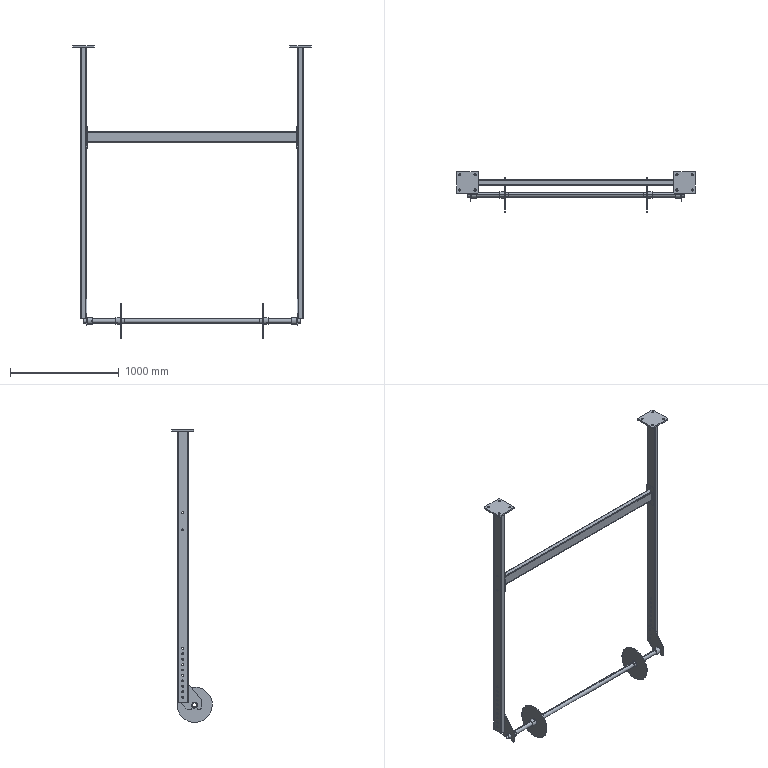Part | SolidWorks | 16 solids | 306 faces | box 2200 x 372.5 x 2697 mm | volume 11177165 mm3 | cylinder 216 | plane 90 | commonest cylinder face diameters 17.5 x104 20 x20 19 x16 8 x12 16 x12 5 x8